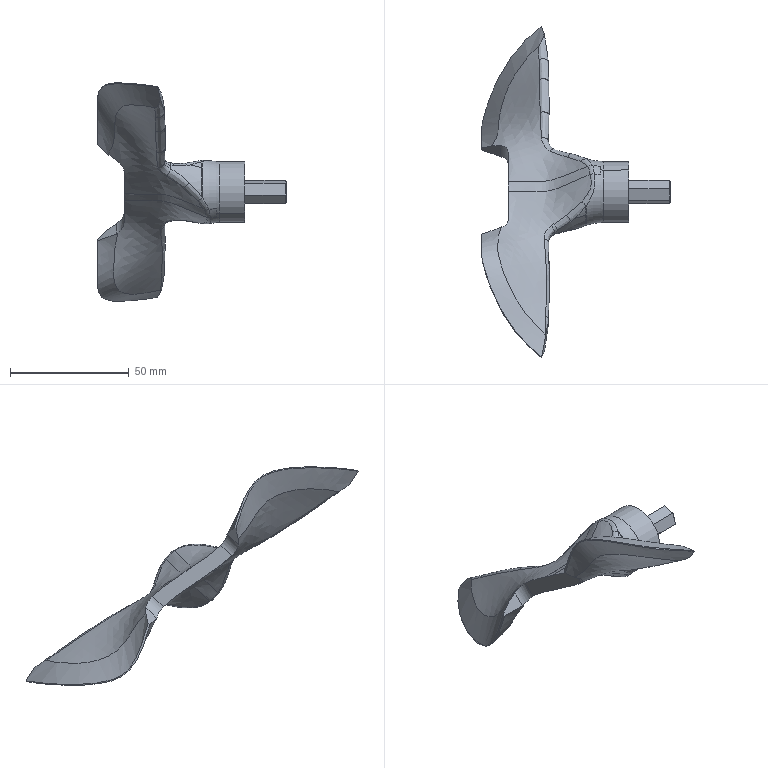Part | SolidWorks | features BaseBody 1 | 1 solid | 89 faces | box 79.382 x 139.536 x 91.87 mm | volume 38859 mm3 | spline 54 | plane 19 | cylinder 10 | cone 4 | torus 2 | commonest cylinder face diameters 226.238 x4 12.135 x2 25.65 x2 1161 x2